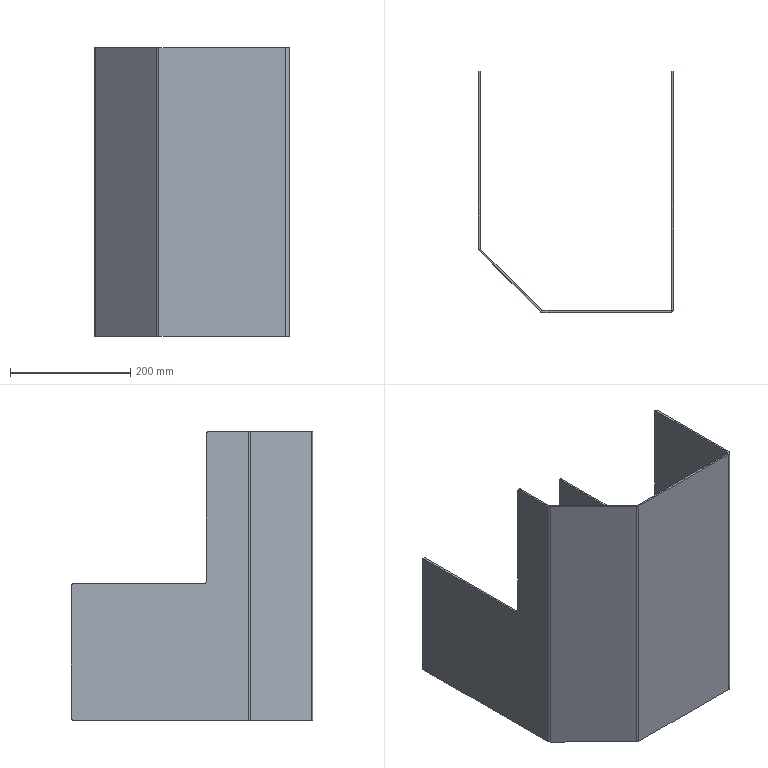Part | SolidWorks | features EdgeFlange 3, FlatPattern 1, SMBaseFlange 1, SheetMetal 1 | 1 solid | 46 faces | box 325 x 402 x 480 mm | volume 1150314 mm3 | plane 28 | cylinder 18 | commonest cylinder face diameters 6 x9 12 x5 8.5 x2 120 x2
STEP:
#1=CARTESIAN_POINT('',(325.,45.,-80.));
#2=VERTEX_POINT('',#1);
#3=CARTESIAN_POINT('',(325.,165.,-80.));
#4=VERTEX_POINT('',#3);
#5=CARTESIAN_POINT('',(325.,105.,-80.));
#6=DIRECTION('',(1.,0.,0.));
#7=DIRECTION('',(0.,1.,0.));
#8=AXIS2_PLACEMENT_3D('',#5,#6,#7);
#9=CIRCLE('',#8,60.);
#10=EDGE_CURVE('',#2,#4,#9,.T.);
#11=ORIENTED_EDGE('',*,*,#10,.T.);
#12=CARTESIAN_POINT('',(322.,165.,-80.));
#13=VERTEX_POINT('',#12);
#14=CARTESIAN_POINT('',(325.,165.,-80.));
#15=DIRECTION('',(-1.,0.,0.));
#16=VECTOR('',#15,1000.);
#17=LINE('',#14,#16);
#18=EDGE_CURVE('',#4,#13,#17,.T.);
#19=ORIENTED_EDGE('',*,*,#18,.T.);
#20=CARTESIAN_POINT('',(322.,45.,-80.));
#21=VERTEX_POINT('',#20);
#22=CARTESIAN_POINT('',(322.,105.,-80.));
#23=DIRECTION('',(1.,0.,0.));
#24=DIRECTION('',(0.,1.,0.));
#25=AXIS2_PLACEMENT_3D('',#22,#23,#24);
#26=CIRCLE('',#25,60.);
#27=EDGE_CURVE('',#21,#13,#26,.T.);
#28=ORIENTED_EDGE('',*,*,#27,.F.);
#29=CARTESIAN_POINT('',(325.,45.,-80.));
#30=DIRECTION('',(-1.,0.,0.));
#31=VECTOR('',#30,1000.);
#32=LINE('',#29,#31);
#33=EDGE_CURVE('',#2,#21,#32,.T.);
#34=ORIENTED_EDGE('',*,*,#33,.F.);
#35=EDGE_LOOP('',(#11,#19,#28,#34));
#36=FACE_OUTER_BOUND('',#35,.T.);
#37=CARTESIAN_POINT('',(325.,105.,-80.));
#38=DIRECTION('',(-1.,0.,0.));
#39=DIRECTION('',(0.,-1.,0.));
#40=AXIS2_PLACEMENT_3D('',#37,#38,#39);
#41=CYLINDRICAL_SURFACE('',#40,60.);
#42=ADVANCED_FACE('',(#36),#41,.F.);
#43=CARTESIAN_POINT('',(325.,25.75,210.));
#44=VERTEX_POINT('',#43);
#45=CARTESIAN_POINT('',(325.,34.25,210.));
#46=VERTEX_POINT('',#45);
#47=CARTESIAN_POINT('',(325.,30.,210.));
#48=DIRECTION('',(1.,0.,0.));
#49=DIRECTION('',(0.,1.,0.));
#50=AXIS2_PLACEMENT_3D('',#47,#48,#49);
#51=CIRCLE('',#50,4.25);
#52=EDGE_CURVE('',#44,#46,#51,.T.);
#53=ORIENTED_EDGE('',*,*,#52,.T.);
#54=CARTESIAN_POINT('',(322.,34.25,210.));
#55=VERTEX_POINT('',#54);
#56=CARTESIAN_POINT('',(325.,34.25,210.));
#57=DIRECTION('',(-1.,0.,0.));
#58=VECTOR('',#57,1000.);
#59=LINE('',#56,#58);
#60=EDGE_CURVE('',#46,#55,#59,.T.);
#61=ORIENTED_EDGE('',*,*,#60,.T.);
#62=CARTESIAN_POINT('',(322.,25.75,210.));
#63=VERTEX_POINT('',#62);
#64=CARTESIAN_POINT('',(322.,30.,210.));
#65=DIRECTION('',(1.,0.,0.));
#66=DIRECTION('',(0.,1.,0.));
#67=AXIS2_PLACEMENT_3D('',#64,#65,#66);
#68=CIRCLE('',#67,4.25);
#69=EDGE_CURVE('',#63,#55,#68,.T.);
#70=ORIENTED_EDGE('',*,*,#69,.F.);
#71=CARTESIAN_POINT('',(325.,25.75,210.));
#72=DIRECTION('',(-1.,0.,0.));
#73=VECTOR('',#72,1000.);
#74=LINE('',#71,#73);
#75=EDGE_CURVE('',#44,#63,#74,.T.);
#76=ORIENTED_EDGE('',*,*,#75,.F.);
#77=EDGE_LOOP('',(#53,#61,#70,#76));
#78=FACE_OUTER_BOUND('',#77,.T.);
#79=CARTESIAN_POINT('',(325.,30.,210.));
#80=DIRECTION('',(-1.,0.,0.));
#81=DIRECTION('',(0.,-1.,0.));
#82=AXIS2_PLACEMENT_3D('',#79,#80,#81);
#83=CYLINDRICAL_SURFACE('',#82,4.25);
#84=ADVANCED_FACE('',(#78),#83,.F.);
#85=CARTESIAN_POINT('',(319.,3.,-240.));
#86=VERTEX_POINT('',#85);
#87=CARTESIAN_POINT('',(107.485,3.,-240.));
#88=VERTEX_POINT('',#87);
#89=CARTESIAN_POINT('',(319.,3.,-240.));
#90=DIRECTION('',(-1.,0.,0.));
#91=VECTOR('',#90,1000.);
#92=LINE('',#89,#91);
#93=EDGE_CURVE('',#86,#88,#92,.T.);
#94=ORIENTED_EDGE('',*,*,#93,.F.);
#95=CARTESIAN_POINT('',(319.,0.,-240.));
#96=VERTEX_POINT('',#95);
#97=CARTESIAN_POINT('',(319.,0.,-240.));
#98=DIRECTION('',(0.,1.,0.));
#99=VECTOR('',#98,1000.);
#100=LINE('',#97,#99);
#101=EDGE_CURVE('',#96,#86,#100,.T.);
#102=ORIENTED_EDGE('',*,*,#101,.F.);
#103=CARTESIAN_POINT('',(107.485,0.,-240.));
#104=VERTEX_POINT('',#103);
#105=CARTESIAN_POINT('',(319.,0.,-240.));
#106=DIRECTION('',(-1.,0.,0.));
#107=VECTOR('',#106,1000.);
#108=LINE('',#105,#107);
#109=EDGE_CURVE('',#96,#104,#108,.T.);
#110=ORIENTED_EDGE('',*,*,#109,.T.);
#111=CARTESIAN_POINT('',(107.485,0.,-240.));
#112=DIRECTION('',(0.,1.,0.));
#113=VECTOR('',#112,1000.);
#114=LINE('',#111,#113);
#115=EDGE_CURVE('',#104,#88,#114,.T.);
#116=ORIENTED_EDGE('',*,*,#115,.T.);
#117=EDGE_LOOP('',(#94,#102,#110,#116));
#118=FACE_OUTER_BOUND('',#117,.T.);
#119=CARTESIAN_POINT('',(319.,0.,-240.));
#120=DIRECTION('',(0.,0.,-1.));
#121=DIRECTION('',(-1.,0.,0.));
#122=AXIS2_PLACEMENT_3D('',#119,#120,#121);
#123=PLANE('',#122);
#124=ADVANCED_FACE('',(#118),#123,.T.);
#125=CARTESIAN_POINT('',(107.485,3.,240.));
#126=VERTEX_POINT('',#125);
#127=CARTESIAN_POINT('',(319.,3.,240.));
#128=VERTEX_POINT('',#127);
#129=CARTESIAN_POINT('',(107.485,3.,240.));
#130=DIRECTION('',(1.,0.,0.));
#131=VECTOR('',#130,1000.);
#132=LINE('',#129,#131);
#133=EDGE_CURVE('',#126,#128,#132,.T.);
#134=ORIENTED_EDGE('',*,*,#133,.F.);
#135=CARTESIAN_POINT('',(107.485,0.,240.));
#136=VERTEX_POINT('',#135);
#137=CARTESIAN_POINT('',(107.485,0.,240.));
#138=DIRECTION('',(0.,1.,0.));
#139=VECTOR('',#138,1000.);
#140=LINE('',#137,#139);
#141=EDGE_CURVE('',#136,#126,#140,.T.);
#142=ORIENTED_EDGE('',*,*,#141,.F.);
#143=CARTESIAN_POINT('',(319.,0.,240.));
#144=VERTEX_POINT('',#143);
#145=CARTESIAN_POINT('',(107.485,0.,240.));
#146=DIRECTION('',(1.,0.,0.));
#147=VECTOR('',#146,1000.);
#148=LINE('',#145,#147);
#149=EDGE_CURVE('',#136,#144,#148,.T.);
#150=ORIENTED_EDGE('',*,*,#149,.T.);
#151=CARTESIAN_POINT('',(319.,0.,240.));
#152=DIRECTION('',(0.,1.,0.));
#153=VECTOR('',#152,1000.);
#154=LINE('',#151,#153);
#155=EDGE_CURVE('',#144,#128,#154,.T.);
#156=ORIENTED_EDGE('',*,*,#155,.T.);
#157=EDGE_LOOP('',(#134,#142,#150,#156));
#158=FACE_OUTER_BOUND('',#157,.T.);
#159=CARTESIAN_POINT('',(107.485,0.,240.));
#160=DIRECTION('',(0.,0.,1.));
#161=DIRECTION('',(1.,0.,0.));
#162=AXIS2_PLACEMENT_3D('',#159,#160,#161);
#163=PLANE('',#162);
#164=ADVANCED_FACE('',(#158),#163,.T.);
#165=ORIENTED_EDGE('',*,*,#109,.F.);
#166=CARTESIAN_POINT('',(319.,0.,240.));
#167=DIRECTION('',(0.,0.,-1.));
#168=VECTOR('',#167,1000.);
#169=LINE('',#166,#168);
#170=EDGE_CURVE('',#144,#96,#169,.T.);
#171=ORIENTED_EDGE('',*,*,#170,.F.);
#172=ORIENTED_EDGE('',*,*,#149,.F.);
#173=CARTESIAN_POINT('',(107.485,0.,-240.));
#174=DIRECTION('',(0.,0.,1.));
#175=VECTOR('',#174,1000.);
#176=LINE('',#173,#175);
#177=EDGE_CURVE('',#104,#136,#176,.T.);
#178=ORIENTED_EDGE('',*,*,#177,.F.);
#179=EDGE_LOOP('',(#165,#171,#172,#178));
#180=FACE_OUTER_BOUND('',#179,.T.);
#181=CARTESIAN_POINT('',(0.,0.,0.));
#182=DIRECTION('',(0.,1.,0.));
#183=DIRECTION('',(0.,0.,1.));
#184=AXIS2_PLACEMENT_3D('',#181,#182,#183);
#185=PLANE('',#184);
#186=ADVANCED_FACE('',(#180),#185,.F.);
#187=ORIENTED_EDGE('',*,*,#93,.T.);
#188=CARTESIAN_POINT('',(107.485,3.,-240.));
#189=DIRECTION('',(0.,0.,1.));
#190=VECTOR('',#189,1000.);
#191=LINE('',#188,#190);
#192=EDGE_CURVE('',#88,#126,#191,.T.);
#193=ORIENTED_EDGE('',*,*,#192,.T.);
#194=ORIENTED_EDGE('',*,*,#133,.T.);
#195=CARTESIAN_POINT('',(319.,3.,240.));
#196=DIRECTION('',(0.,0.,-1.));
#197=VECTOR('',#196,1000.);
#198=LINE('',#195,#197);
#199=EDGE_CURVE('',#128,#86,#198,.T.);
#200=ORIENTED_EDGE('',*,*,#199,.T.);
#201=EDGE_LOOP('',(#187,#193,#194,#200));
#202=FACE_OUTER_BOUND('',#201,.T.);
#203=CARTESIAN_POINT('',(0.,3.,0.));
#204=DIRECTION('',(0.,1.,0.));
#205=DIRECTION('',(0.,0.,1.));
#206=AXIS2_PLACEMENT_3D('',#203,#204,#205);
#207=PLANE('',#206);
#208=ADVANCED_FACE('',(#202),#207,.T.);
#209=CARTESIAN_POINT('',(105.364,3.879,-240.));
#210=VERTEX_POINT('',#209);
#211=CARTESIAN_POINT('',(103.243,1.757,-240.));
#212=VERTEX_POINT('',#211);
#213=CARTESIAN_POINT('',(103.243,1.757,-240.));
#214=DIRECTION('',(-0.7071,-0.7071,0.));
#215=VECTOR('',#214,1000.);
#216=LINE('',#213,#215);
#217=EDGE_CURVE('',#210,#212,#216,.T.);
#218=ORIENTED_EDGE('',*,*,#217,.F.);
#219=CARTESIAN_POINT('',(107.485,6.,-240.));
#220=DIRECTION('',(0.,0.,-1.));
#221=DIRECTION('',(1.,0.,0.));
#222=AXIS2_PLACEMENT_3D('',#219,#220,#221);
#223=CIRCLE('',#222,3.);
#224=EDGE_CURVE('',#88,#210,#223,.T.);
#225=ORIENTED_EDGE('',*,*,#224,.F.);
#226=ORIENTED_EDGE('',*,*,#115,.F.);
#227=CARTESIAN_POINT('',(107.485,6.,-240.));
#228=DIRECTION('',(0.,0.,-1.));
#229=DIRECTION('',(1.,0.,0.));
#230=AXIS2_PLACEMENT_3D('',#227,#228,#229);
#231=CIRCLE('',#230,6.);
#232=EDGE_CURVE('',#104,#212,#231,.T.);
#233=ORIENTED_EDGE('',*,*,#232,.T.);
#234=EDGE_LOOP('',(#218,#225,#226,#233));
#235=FACE_OUTER_BOUND('',#234,.T.);
#236=CARTESIAN_POINT('',(107.485,6.,-240.));
#237=DIRECTION('',(0.,0.,-1.));
#238=DIRECTION('',(-1.,0.,0.));
#239=AXIS2_PLACEMENT_3D('',#236,#237,#238);
#240=PLANE('',#239);
#241=ADVANCED_FACE('',(#235),#240,.T.);
#242=CARTESIAN_POINT('',(105.364,3.879,240.));
#243=VERTEX_POINT('',#242);
#244=CARTESIAN_POINT('',(107.485,6.,240.));
#245=DIRECTION('',(0.,0.,1.));
#246=DIRECTION('',(1.,0.,0.));
#247=AXIS2_PLACEMENT_3D('',#244,#245,#246);
#248=CIRCLE('',#247,3.);
#249=EDGE_CURVE('',#243,#126,#248,.T.);
#250=ORIENTED_EDGE('',*,*,#249,.F.);
#251=CARTESIAN_POINT('',(103.243,1.757,240.));
#252=VERTEX_POINT('',#251);
#253=CARTESIAN_POINT('',(105.364,3.879,240.));
#254=DIRECTION('',(-0.7071,-0.7071,0.));
#255=VECTOR('',#254,1000.);
#256=LINE('',#253,#255);
#257=EDGE_CURVE('',#243,#252,#256,.T.);
#258=ORIENTED_EDGE('',*,*,#257,.T.);
#259=CARTESIAN_POINT('',(107.485,6.,240.));
#260=DIRECTION('',(0.,0.,1.));
#261=DIRECTION('',(1.,0.,0.));
#262=AXIS2_PLACEMENT_3D('',#259,#260,#261);
#263=CIRCLE('',#262,6.);
#264=EDGE_CURVE('',#252,#136,#263,.T.);
#265=ORIENTED_EDGE('',*,*,#264,.T.);
#266=ORIENTED_EDGE('',*,*,#141,.T.);
#267=EDGE_LOOP('',(#250,#258,#265,#266));
#268=FACE_OUTER_BOUND('',#267,.T.);
#269=CARTESIAN_POINT('',(107.485,6.,240.));
#270=DIRECTION('',(0.,0.,-1.));
#271=DIRECTION('',(-1.,0.,0.));
#272=AXIS2_PLACEMENT_3D('',#269,#270,#271);
#273=PLANE('',#272);
#274=ADVANCED_FACE('',(#268),#273,.F.);
#275=ORIENTED_EDGE('',*,*,#177,.T.);
#276=ORIENTED_EDGE('',*,*,#264,.F.);
#277=CARTESIAN_POINT('',(103.243,1.757,-240.));
#278=DIRECTION('',(0.,0.,-1.));
#279=VECTOR('',#278,1000.);
#280=LINE('',#277,#279);
#281=EDGE_CURVE('',#252,#212,#280,.T.);
#282=ORIENTED_EDGE('',*,*,#281,.T.);
#283=ORIENTED_EDGE('',*,*,#232,.F.);
#284=EDGE_LOOP('',(#275,#276,#282,#283));
#285=FACE_OUTER_BOUND('',#284,.T.);
#286=CARTESIAN_POINT('',(107.485,6.,240.));
#287=DIRECTION('',(0.,0.,1.));
#288=DIRECTION('',(-0.7071,-0.7071,0.));
#289=AXIS2_PLACEMENT_3D('',#286,#287,#288);
#290=CYLINDRICAL_SURFACE('',#289,6.);
#291=ADVANCED_FACE('',(#285),#290,.T.);
#292=ORIENTED_EDGE('',*,*,#192,.F.);
#293=ORIENTED_EDGE('',*,*,#224,.T.);
#294=CARTESIAN_POINT('',(105.364,3.879,-240.));
#295=DIRECTION('',(0.,0.,1.));
#296=VECTOR('',#295,1000.);
#297=LINE('',#294,#296);
#298=EDGE_CURVE('',#210,#243,#297,.T.);
#299=ORIENTED_EDGE('',*,*,#298,.T.);
#300=ORIENTED_EDGE('',*,*,#249,.T.);
#301=EDGE_LOOP('',(#292,#293,#299,#300));
#302=FACE_OUTER_BOUND('',#301,.T.);
#303=CARTESIAN_POINT('',(107.485,6.,240.));
#304=DIRECTION('',(0.,0.,1.));
#305=DIRECTION('',(-0.7071,-0.7071,0.));
#306=AXIS2_PLACEMENT_3D('',#303,#304,#305);
#307=CYLINDRICAL_SURFACE('',#306,3.);
#308=ADVANCED_FACE('',(#302),#307,.F.);
#309=ORIENTED_EDGE('',*,*,#257,.F.);
#310=CARTESIAN_POINT('',(3.879,105.364,240.));
#311=VERTEX_POINT('',#310);
#312=CARTESIAN_POINT('',(3.879,105.364,240.));
#313=DIRECTION('',(-0.7071,0.7071,0.));
#314=VECTOR('',#313,1000.);
#315=LINE('',#312,#314);
#316=EDGE_CURVE('',#243,#311,#315,.T.);
#317=ORIENTED_EDGE('',*,*,#316,.T.);
#318=CARTESIAN_POINT('',(1.757,103.243,240.));
#319=VERTEX_POINT('',#318);
#320=CARTESIAN_POINT('',(1.757,103.243,240.));
#321=DIRECTION('',(0.7071,0.7071,0.));
#322=VECTOR('',#321,1000.);
#323=LINE('',#320,#322);
#324=EDGE_CURVE('',#319,#311,#323,.T.);
#325=ORIENTED_EDGE('',*,*,#324,.F.);
#326=CARTESIAN_POINT('',(51.879,53.121,240.));
#327=DIRECTION('',(-0.7071,0.7071,0.));
#328=VECTOR('',#327,1000.);
#329=LINE('',#326,#328);
#330=EDGE_CURVE('',#252,#319,#329,.T.);
#331=ORIENTED_EDGE('',*,*,#330,.F.);
#332=EDGE_LOOP('',(#309,#317,#325,#331));
#333=FACE_OUTER_BOUND('',#332,.T.);
#334=CARTESIAN_POINT('',(1.757,103.243,240.));
#335=DIRECTION('',(0.,0.,-1.));
#336=DIRECTION('',(-1.,0.,0.));
#337=AXIS2_PLACEMENT_3D('',#334,#335,#336);
#338=PLANE('',#337);
#339=ADVANCED_FACE('',(#333),#338,.F.);
#340=ORIENTED_EDGE('',*,*,#217,.T.);
#341=CARTESIAN_POINT('',(1.757,103.243,-240.));
#342=VERTEX_POINT('',#341);
#343=CARTESIAN_POINT('',(51.879,53.121,-240.));
#344=DIRECTION('',(0.7071,-0.7071,0.));
#345=VECTOR('',#344,1000.);
#346=LINE('',#343,#345);
#347=EDGE_CURVE('',#342,#212,#346,.T.);
#348=ORIENTED_EDGE('',*,*,#347,.F.);
#349=CARTESIAN_POINT('',(3.879,105.364,-240.));
#350=VERTEX_POINT('',#349);
#351=CARTESIAN_POINT('',(1.757,103.243,-240.));
#352=DIRECTION('',(0.7071,0.7071,0.));
#353=VECTOR('',#352,1000.);
#354=LINE('',#351,#353);
#355=EDGE_CURVE('',#342,#350,#354,.T.);
#356=ORIENTED_EDGE('',*,*,#355,.T.);
#357=CARTESIAN_POINT('',(106.243,3.,-240.));
#358=DIRECTION('',(0.7071,-0.7071,0.));
#359=VECTOR('',#358,1000.);
#360=LINE('',#357,#359);
#361=EDGE_CURVE('',#350,#210,#360,.T.);
#362=ORIENTED_EDGE('',*,*,#361,.T.);
#363=EDGE_LOOP('',(#340,#348,#356,#362));
#364=FACE_OUTER_BOUND('',#363,.T.);
#365=CARTESIAN_POINT('',(104.121,0.8787,-240.));
#366=DIRECTION('',(0.,0.,1.));
#367=DIRECTION('',(1.,0.,0.));
#368=AXIS2_PLACEMENT_3D('',#365,#366,#367);
#369=PLANE('',#368);
#370=ADVANCED_FACE('',(#364),#369,.F.);
#371=ORIENTED_EDGE('',*,*,#281,.F.);
#372=ORIENTED_EDGE('',*,*,#330,.T.);
#373=CARTESIAN_POINT('',(1.757,103.243,0.));
#374=DIRECTION('',(0.,0.,-1.));
#375=VECTOR('',#374,1000.);
#376=LINE('',#373,#375);
#377=EDGE_CURVE('',#319,#342,#376,.T.);
#378=ORIENTED_EDGE('',*,*,#377,.T.);
#379=ORIENTED_EDGE('',*,*,#347,.T.);
#380=EDGE_LOOP('',(#371,#372,#378,#379));
#381=FACE_OUTER_BOUND('',#380,.T.);
#382=CARTESIAN_POINT('',(51.879,53.121,0.));
#383=DIRECTION('',(0.7071,0.7071,0.));
#384=DIRECTION('',(-0.7071,0.7071,0.));
#385=AXIS2_PLACEMENT_3D('',#382,#383,#384);
#386=PLANE('',#385);
#387=ADVANCED_FACE('',(#381),#386,.F.);
#388=ORIENTED_EDGE('',*,*,#316,.F.);
#389=ORIENTED_EDGE('',*,*,#298,.F.);
#390=ORIENTED_EDGE('',*,*,#361,.F.);
#391=CARTESIAN_POINT('',(3.879,105.364,-240.));
#392=DIRECTION('',(0.,0.,-1.));
#393=VECTOR('',#392,1000.);
#394=LINE('',#391,#393);
#395=EDGE_CURVE('',#311,#350,#394,.T.);
#396=ORIENTED_EDGE('',*,*,#395,.F.);
#397=EDGE_LOOP('',(#388,#389,#390,#396));
#398=FACE_OUTER_BOUND('',#397,.T.);
#399=CARTESIAN_POINT('',(54.,55.243,0.));
#400=DIRECTION('',(0.7071,0.7071,0.));
#401=DIRECTION('',(-0.7071,0.7071,0.));
#402=AXIS2_PLACEMENT_3D('',#399,#400,#401);
#403=PLANE('',#402);
#404=ADVANCED_FACE('',(#398),#403,.T.);
#405=CARTESIAN_POINT('',(322.,6.,240.));
#406=VERTEX_POINT('',#405);
#407=CARTESIAN_POINT('',(325.,6.,240.));
#408=VERTEX_POINT('',#407);
#409=CARTESIAN_POINT('',(325.,6.,240.));
#410=DIRECTION('',(1.,0.,0.));
#411=VECTOR('',#410,1000.);
#412=LINE('',#409,#411);
#413=EDGE_CURVE('',#406,#408,#412,.T.);
#414=ORIENTED_EDGE('',*,*,#413,.F.);
#415=CARTESIAN_POINT('',(319.,6.,240.));
#416=DIRECTION('',(0.,0.,1.));
#417=DIRECTION('',(-1.,0.,0.));
#418=AXIS2_PLACEMENT_3D('',#415,#416,#417);
#419=CIRCLE('',#418,3.);
#420=EDGE_CURVE('',#128,#406,#419,.T.);
#421=ORIENTED_EDGE('',*,*,#420,.F.);
#422=ORIENTED_EDGE('',*,*,#155,.F.);
#423=CARTESIAN_POINT('',(319.,6.,240.));
#424=DIRECTION('',(0.,0.,1.));
#425=DIRECTION('',(-1.,0.,0.));
#426=AXIS2_PLACEMENT_3D('',#423,#424,#425);
#427=CIRCLE('',#426,6.);
#428=EDGE_CURVE('',#144,#408,#427,.T.);
#429=ORIENTED_EDGE('',*,*,#428,.T.);
#430=EDGE_LOOP('',(#414,#421,#422,#429));
#431=FACE_OUTER_BOUND('',#430,.T.);
#432=CARTESIAN_POINT('',(319.,6.,240.));
#433=DIRECTION('',(0.,0.,1.));
#434=DIRECTION('',(1.,0.,0.));
#435=AXIS2_PLACEMENT_3D('',#432,#433,#434);
#436=PLANE('',#435);
#437=ADVANCED_FACE('',(#431),#436,.T.);
#438=CARTESIAN_POINT('',(322.,6.,-240.));
#439=VERTEX_POINT('',#438);
#440=CARTESIAN_POINT('',(319.,6.,-240.));
#441=DIRECTION('',(0.,0.,-1.));
#442=DIRECTION('',(-1.,0.,0.));
#443=AXIS2_PLACEMENT_3D('',#440,#441,#442);
#444=CIRCLE('',#443,3.);
#445=EDGE_CURVE('',#439,#86,#444,.T.);
#446=ORIENTED_EDGE('',*,*,#445,.F.);
#447=CARTESIAN_POINT('',(325.,6.,-240.));
#448=VERTEX_POINT('',#447);
#449=CARTESIAN_POINT('',(322.,6.,-240.));
#450=DIRECTION('',(1.,0.,0.));
#451=VECTOR('',#450,1000.);
#452=LINE('',#449,#451);
#453=EDGE_CURVE('',#439,#448,#452,.T.);
#454=ORIENTED_EDGE('',*,*,#453,.T.);
#455=CARTESIAN_POINT('',(319.,6.,-240.));
#456=DIRECTION('',(0.,0.,-1.));
#457=DIRECTION('',(-1.,0.,0.));
#458=AXIS2_PLACEMENT_3D('',#455,#456,#457);
#459=CIRCLE('',#458,6.);
#460=EDGE_CURVE('',#448,#96,#459,.T.);
#461=ORIENTED_EDGE('',*,*,#460,.T.);
#462=ORIENTED_EDGE('',*,*,#101,.T.);
#463=EDGE_LOOP('',(#446,#454,#461,#462));
#464=FACE_OUTER_BOUND('',#463,.T.);
#465=CARTESIAN_POINT('',(319.,6.,-240.));
#466=DIRECTION('',(0.,0.,1.));
#467=DIRECTION('',(1.,0.,0.));
#468=AXIS2_PLACEMENT_3D('',#465,#466,#467);
#469=PLANE('',#468);
#470=ADVANCED_FACE('',(#464),#469,.F.);
#471=ORIENTED_EDGE('',*,*,#170,.T.);
#472=ORIENTED_EDGE('',*,*,#460,.F.);
#473=CARTESIAN_POINT('',(325.,6.,237.));
#474=DIRECTION('',(0.,0.,-1.));
#475=VECTOR('',#474,1000.);
#476=LINE('',#473,#475);
#477=EDGE_CURVE('',#408,#448,#476,.T.);
#478=ORIENTED_EDGE('',*,*,#477,.F.);
#479=ORIENTED_EDGE('',*,*,#428,.F.);
#480=EDGE_LOOP('',(#471,#472,#478,#479));
#481=FACE_OUTER_BOUND('',#480,.T.);
#482=CARTESIAN_POINT('',(319.,6.,-240.));
#483=DIRECTION('',(0.,0.,-1.));
#484=DIRECTION('',(1.,0.,0.));
#485=AXIS2_PLACEMENT_3D('',#482,#483,#484);
#486=CYLINDRICAL_SURFACE('',#485,6.);
#487=ADVANCED_FACE('',(#481),#486,.T.);
#488=ORIENTED_EDGE('',*,*,#199,.F.);
#489=ORIENTED_EDGE('',*,*,#420,.T.);
#490=CARTESIAN_POINT('',(322.,6.,240.));
#491=DIRECTION('',(0.,0.,-1.));
#492=VECTOR('',#491,1000.);
#493=LINE('',#490,#492);
#494=EDGE_CURVE('',#406,#439,#493,.T.);
#495=ORIENTED_EDGE('',*,*,#494,.T.);
#496=ORIENTED_EDGE('',*,*,#445,.T.);
#497=EDGE_LOOP('',(#488,#489,#495,#496));
#498=FACE_OUTER_BOUND('',#497,.T.);
#499=CARTESIAN_POINT('',(319.,6.,-240.));
#500=DIRECTION('',(0.,0.,-1.));
#501=DIRECTION('',(1.,0.,0.));
#502=AXIS2_PLACEMENT_3D('',#499,#500,#501);
#503=CYLINDRICAL_SURFACE('',#502,3.);
#504=ADVANCED_FACE('',(#498),#503,.F.);
#505=ORIENTED_EDGE('',*,*,#52,.F.);
#506=CARTESIAN_POINT('',(325.,30.,210.));
#507=DIRECTION('',(1.,0.,0.));
#508=DIRECTION('',(0.,1.,0.));
#509=AXIS2_PLACEMENT_3D('',#506,#507,#508);
#510=CIRCLE('',#509,4.25);
#511=EDGE_CURVE('',#46,#44,#510,.T.);
#512=ORIENTED_EDGE('',*,*,#511,.F.);
#513=EDGE_LOOP('',(#505,#512));
#514=FACE_BOUND('',#513,.T.);
#515=ORIENTED_EDGE('',*,*,#10,.F.);
#516=CARTESIAN_POINT('',(325.,105.,-80.));
#517=DIRECTION('',(1.,0.,0.));
#518=DIRECTION('',(0.,1.,0.));
#519=AXIS2_PLACEMENT_3D('',#516,#517,#518);
#520=CIRCLE('',#519,60.);
#521=EDGE_CURVE('',#4,#2,#520,.T.);
#522=ORIENTED_EDGE('',*,*,#521,.F.);
#523=EDGE_LOOP('',(#515,#522));
#524=FACE_BOUND('',#523,.T.);
#525=CARTESIAN_POINT('',(325.,174.,240.));
#526=VERTEX_POINT('',#525);
#527=CARTESIAN_POINT('',(325.,174.,240.));
#528=DIRECTION('',(0.,-1.,0.));
#529=VECTOR('',#528,1000.);
#530=LINE('',#527,#529);
#531=EDGE_CURVE('',#526,#408,#530,.T.);
#532=ORIENTED_EDGE('',*,*,#531,.T.);
#533=ORIENTED_EDGE('',*,*,#477,.T.);
#534=CARTESIAN_POINT('',(325.,399.,-240.));
#535=VERTEX_POINT('',#534);
#536=CARTESIAN_POINT('',(325.,174.,-240.));
#537=DIRECTION('',(0.,1.,0.));
#538=VECTOR('',#537,1000.);
#539=LINE('',#536,#538);
#540=EDGE_CURVE('',#448,#535,#539,.T.);
#541=ORIENTED_EDGE('',*,*,#540,.T.);
#542=CARTESIAN_POINT('',(325.,402.,-237.));
#543=VERTEX_POINT('',#542);
#544=CARTESIAN_POINT('',(325.,399.,-237.));
#545=DIRECTION('',(1.,0.,0.));
#546=DIRECTION('',(0.,1.,0.));
#547=AXIS2_PLACEMENT_3D('',#544,#545,#546);
#548=CIRCLE('',#547,3.);
#549=EDGE_CURVE('',#535,#543,#548,.T.);
#550=ORIENTED_EDGE('',*,*,#549,.T.);
#551=CARTESIAN_POINT('',(325.,402.,-16.));
#552=VERTEX_POINT('',#551);
#553=CARTESIAN_POINT('',(325.,402.,237.));
#554=DIRECTION('',(0.,0.,1.));
#555=VECTOR('',#554,1000.);
#556=LINE('',#553,#555);
#557=EDGE_CURVE('',#543,#552,#556,.T.);
#558=ORIENTED_EDGE('',*,*,#557,.T.);
#559=CARTESIAN_POINT('',(325.,399.,-13.));
#560=VERTEX_POINT('',#559);
#561=CARTESIAN_POINT('',(325.,399.,-16.));
#562=DIRECTION('',(1.,0.,0.));
#563=DIRECTION('',(0.,1.,0.));
#564=AXIS2_PLACEMENT_3D('',#561,#562,#563);
#565=CIRCLE('',#564,3.);
#566=EDGE_CURVE('',#552,#560,#565,.T.);
#567=ORIENTED_EDGE('',*,*,#566,.T.);
#568=CARTESIAN_POINT('',(325.,183.,-13.));
#569=VERTEX_POINT('',#568);
#570=CARTESIAN_POINT('',(325.,174.,-13.));
#571=DIRECTION('',(0.,-1.,0.));
#572=VECTOR('',#571,1000.);
#573=LINE('',#570,#572);
#574=EDGE_CURVE('',#560,#569,#573,.T.);
#575=ORIENTED_EDGE('',*,*,#574,.T.);
#576=CARTESIAN_POINT('',(325.,177.,-7.));
#577=VERTEX_POINT('',#576);
#578=CARTESIAN_POINT('',(325.,183.,-7.));
#579=DIRECTION('',(-1.,0.,0.));
#580=DIRECTION('',(0.,1.,0.));
#581=AXIS2_PLACEMENT_3D('',#578,#579,#580);
#582=CIRCLE('',#581,6.);
#583=EDGE_CURVE('',#569,#577,#582,.T.);
#584=ORIENTED_EDGE('',*,*,#583,.T.);
#585=CARTESIAN_POINT('',(325.,177.,237.));
#586=VERTEX_POINT('',#585);
#587=CARTESIAN_POINT('',(325.,177.,237.));
#588=DIRECTION('',(0.,0.,1.));
#589=VECTOR('',#588,1000.);
#590=LINE('',#587,#589);
#591=EDGE_CURVE('',#577,#586,#590,.T.);
#592=ORIENTED_EDGE('',*,*,#591,.T.);
#593=CARTESIAN_POINT('',(325.,174.,237.));
#594=DIRECTION('',(1.,0.,0.));
#595=DIRECTION('',(0.,1.,0.));
#596=AXIS2_PLACEMENT_3D('',#593,#594,#595);
#597=CIRCLE('',#596,3.);
#598=EDGE_CURVE('',#586,#526,#597,.T.);
#599=ORIENTED_EDGE('',*,*,#598,.T.);
#600=EDGE_LOOP('',(#532,#533,#541,#550,#558,#567,#575,#584,#592,#599));
#601=FACE_OUTER_BOUND('',#600,.T.);
#602=CARTESIAN_POINT('',(325.,174.,237.));
#603=DIRECTION('',(1.,0.,0.));
#604=DIRECTION('',(0.,1.,0.));
#605=AXIS2_PLACEMENT_3D('',#602,#603,#604);
#606=PLANE('',#605);
#607=ADVANCED_FACE('',(#514,#524,#601),#606,.T.);
#608=ORIENTED_EDGE('',*,*,#27,.T.);
#609=CARTESIAN_POINT('',(322.,105.,-80.));
#610=DIRECTION('',(1.,0.,0.));
#611=DIRECTION('',(0.,1.,0.));
#612=AXIS2_PLACEMENT_3D('',#609,#610,#611);
#613=CIRCLE('',#612,60.);
#614=EDGE_CURVE('',#13,#21,#613,.T.);
#615=ORIENTED_EDGE('',*,*,#614,.T.);
#616=EDGE_LOOP('',(#608,#615));
#617=FACE_BOUND('',#616,.T.);
#618=ORIENTED_EDGE('',*,*,#69,.T.);
#619=CARTESIAN_POINT('',(322.,30.,210.));
#620=DIRECTION('',(1.,0.,0.));
#621=DIRECTION('',(0.,1.,0.));
#622=AXIS2_PLACEMENT_3D('',#619,#620,#621);
#623=CIRCLE('',#622,4.25);
#624=EDGE_CURVE('',#55,#63,#623,.T.);
#625=ORIENTED_EDGE('',*,*,#624,.T.);
#626=EDGE_LOOP('',(#618,#625));
#627=FACE_BOUND('',#626,.T.);
#628=ORIENTED_EDGE('',*,*,#494,.F.);
#629=CARTESIAN_POINT('',(322.,174.,240.));
#630=VERTEX_POINT('',#629);
#631=CARTESIAN_POINT('',(322.,3.,240.));
#632=DIRECTION('',(0.,-1.,0.));
#633=VECTOR('',#632,1000.);
#634=LINE('',#631,#633);
#635=EDGE_CURVE('',#630,#406,#634,.T.);
#636=ORIENTED_EDGE('',*,*,#635,.F.);
#637=CARTESIAN_POINT('',(322.,177.,237.));
#638=VERTEX_POINT('',#637);
#639=CARTESIAN_POINT('',(322.,174.,237.));
#640=DIRECTION('',(1.,0.,0.));
#641=DIRECTION('',(0.,1.,0.));
#642=AXIS2_PLACEMENT_3D('',#639,#640,#641);
#643=CIRCLE('',#642,3.);
#644=EDGE_CURVE('',#638,#630,#643,.T.);
#645=ORIENTED_EDGE('',*,*,#644,.F.);
#646=CARTESIAN_POINT('',(322.,177.,-7.));
#647=VERTEX_POINT('',#646);
#648=CARTESIAN_POINT('',(322.,177.,237.));
#649=DIRECTION('',(0.,0.,1.));
#650=VECTOR('',#649,1000.);
#651=LINE('',#648,#650);
#652=EDGE_CURVE('',#647,#638,#651,.T.);
#653=ORIENTED_EDGE('',*,*,#652,.F.);
#654=CARTESIAN_POINT('',(322.,183.,-13.));
#655=VERTEX_POINT('',#654);
#656=CARTESIAN_POINT('',(322.,183.,-7.));
#657=DIRECTION('',(-1.,0.,0.));
#658=DIRECTION('',(0.,1.,0.));
#659=AXIS2_PLACEMENT_3D('',#656,#657,#658);
#660=CIRCLE('',#659,6.);
#661=EDGE_CURVE('',#655,#647,#660,.T.);
#662=ORIENTED_EDGE('',*,*,#661,.F.);
#663=CARTESIAN_POINT('',(322.,399.,-13.));
#664=VERTEX_POINT('',#663);
#665=CARTESIAN_POINT('',(322.,183.,-13.));
#666=DIRECTION('',(0.,-1.,0.));
#667=VECTOR('',#666,1000.);
#668=LINE('',#665,#667);
#669=EDGE_CURVE('',#664,#655,#668,.T.);
#670=ORIENTED_EDGE('',*,*,#669,.F.);
#671=CARTESIAN_POINT('',(322.,402.,-16.));
#672=VERTEX_POINT('',#671);
#673=CARTESIAN_POINT('',(322.,399.,-16.));
#674=DIRECTION('',(1.,0.,0.));
#675=DIRECTION('',(0.,1.,0.));
#676=AXIS2_PLACEMENT_3D('',#673,#674,#675);
#677=CIRCLE('',#676,3.);
#678=EDGE_CURVE('',#672,#664,#677,.T.);
#679=ORIENTED_EDGE('',*,*,#678,.F.);
#680=CARTESIAN_POINT('',(322.,402.,-237.));
#681=VERTEX_POINT('',#680);
#682=CARTESIAN_POINT('',(322.,402.,-16.));
#683=DIRECTION('',(0.,0.,1.));
#684=VECTOR('',#683,1000.);
#685=LINE('',#682,#684);
#686=EDGE_CURVE('',#681,#672,#685,.T.);
#687=ORIENTED_EDGE('',*,*,#686,.F.);
#688=CARTESIAN_POINT('',(322.,399.,-240.));
#689=VERTEX_POINT('',#688);
#690=CARTESIAN_POINT('',(322.,399.,-237.));
#691=DIRECTION('',(1.,0.,0.));
#692=DIRECTION('',(0.,1.,0.));
#693=AXIS2_PLACEMENT_3D('',#690,#691,#692);
#694=CIRCLE('',#693,3.);
#695=EDGE_CURVE('',#689,#681,#694,.T.);
#696=ORIENTED_EDGE('',*,*,#695,.F.);
#697=CARTESIAN_POINT('',(322.,399.,-240.));
#698=DIRECTION('',(0.,1.,0.));
#699=VECTOR('',#698,1000.);
#700=LINE('',#697,#699);
#701=EDGE_CURVE('',#439,#689,#700,.T.);
#702=ORIENTED_EDGE('',*,*,#701,.F.);
#703=EDGE_LOOP('',(#628,#636,#645,#653,#662,#670,#679,#687,#696,#702));
#704=FACE_OUTER_BOUND('',#703,.T.);
#705=CARTESIAN_POINT('',(322.,174.,237.));
#706=DIRECTION('',(1.,0.,0.));
#707=DIRECTION('',(0.,1.,0.));
#708=AXIS2_PLACEMENT_3D('',#705,#706,#707);
#709=PLANE('',#708);
#710=ADVANCED_FACE('',(#617,#627,#704),#709,.F.);
#711=ORIENTED_EDGE('',*,*,#453,.F.);
#712=ORIENTED_EDGE('',*,*,#701,.T.);
#713=CARTESIAN_POINT('',(325.,399.,-240.));
#714=DIRECTION('',(-1.,0.,0.));
#715=VECTOR('',#714,1000.);
#716=LINE('',#713,#715);
#717=EDGE_CURVE('',#535,#689,#716,.T.);
#718=ORIENTED_EDGE('',*,*,#717,.F.);
#719=ORIENTED_EDGE('',*,*,#540,.F.);
#720=EDGE_LOOP('',(#711,#712,#718,#719));
#721=FACE_OUTER_BOUND('',#720,.T.);
#722=CARTESIAN_POINT('',(325.,399.,-240.));
#723=DIRECTION('',(0.,0.,1.));
#724=DIRECTION('',(1.,0.,0.));
#725=AXIS2_PLACEMENT_3D('',#722,#723,#724);
#726=PLANE('',#725);
#727=ADVANCED_FACE('',(#721),#726,.F.);
#728=ORIENTED_EDGE('',*,*,#413,.T.);
#729=ORIENTED_EDGE('',*,*,#531,.F.);
#730=CARTESIAN_POINT('',(325.,174.,240.));
#731=DIRECTION('',(-1.,0.,0.));
#732=VECTOR('',#731,1000.);
#733=LINE('',#730,#732);
#734=EDGE_CURVE('',#526,#630,#733,.T.);
#735=ORIENTED_EDGE('',*,*,#734,.T.);
#736=ORIENTED_EDGE('',*,*,#635,.T.);
#737=EDGE_LOOP('',(#728,#729,#735,#736));
#738=FACE_OUTER_BOUND('',#737,.T.);
#739=CARTESIAN_POINT('',(325.,3.,240.));
#740=DIRECTION('',(0.,0.,-1.));
#741=DIRECTION('',(-1.,0.,0.));
#742=AXIS2_PLACEMENT_3D('',#739,#740,#741);
#743=PLANE('',#742);
#744=ADVANCED_FACE('',(#738),#743,.F.);
#745=ORIENTED_EDGE('',*,*,#695,.T.);
#746=CARTESIAN_POINT('',(325.,402.,-237.));
#747=DIRECTION('',(-1.,0.,0.));
#748=VECTOR('',#747,1000.);
#749=LINE('',#746,#748);
#750=EDGE_CURVE('',#543,#681,#749,.T.);
#751=ORIENTED_EDGE('',*,*,#750,.F.);
#752=ORIENTED_EDGE('',*,*,#549,.F.);
#753=ORIENTED_EDGE('',*,*,#717,.T.);
#754=EDGE_LOOP('',(#745,#751,#752,#753));
#755=FACE_OUTER_BOUND('',#754,.T.);
#756=CARTESIAN_POINT('',(325.,399.,-237.));
#757=DIRECTION('',(-1.,0.,0.));
#758=DIRECTION('',(0.,-1.,0.));
#759=AXIS2_PLACEMENT_3D('',#756,#757,#758);
#760=CYLINDRICAL_SURFACE('',#759,3.);
#761=ADVANCED_FACE('',(#755),#760,.T.);
#762=ORIENTED_EDGE('',*,*,#686,.T.);
#763=CARTESIAN_POINT('',(325.,402.,-16.));
#764=DIRECTION('',(-1.,0.,0.));
#765=VECTOR('',#764,1000.);
#766=LINE('',#763,#765);
#767=EDGE_CURVE('',#552,#672,#766,.T.);
#768=ORIENTED_EDGE('',*,*,#767,.F.);
#769=ORIENTED_EDGE('',*,*,#557,.F.);
#770=ORIENTED_EDGE('',*,*,#750,.T.);
#771=EDGE_LOOP('',(#762,#768,#769,#770));
#772=FACE_OUTER_BOUND('',#771,.T.);
#773=CARTESIAN_POINT('',(325.,402.,-16.));
#774=DIRECTION('',(0.,-1.,0.));
#775=DIRECTION('',(1.,0.,0.));
#776=AXIS2_PLACEMENT_3D('',#773,#774,#775);
#777=PLANE('',#776);
#778=ADVANCED_FACE('',(#772),#777,.F.);
#779=ORIENTED_EDGE('',*,*,#678,.T.);
#780=CARTESIAN_POINT('',(325.,399.,-13.));
#781=DIRECTION('',(-1.,0.,0.));
#782=VECTOR('',#781,1000.);
#783=LINE('',#780,#782);
#784=EDGE_CURVE('',#560,#664,#783,.T.);
#785=ORIENTED_EDGE('',*,*,#784,.F.);
#786=ORIENTED_EDGE('',*,*,#566,.F.);
#787=ORIENTED_EDGE('',*,*,#767,.T.);
#788=EDGE_LOOP('',(#779,#785,#786,#787));
#789=FACE_OUTER_BOUND('',#788,.T.);
#790=CARTESIAN_POINT('',(325.,399.,-16.));
#791=DIRECTION('',(-1.,0.,0.));
#792=DIRECTION('',(0.,-1.,0.));
#793=AXIS2_PLACEMENT_3D('',#790,#791,#792);
#794=CYLINDRICAL_SURFACE('',#793,3.);
#795=ADVANCED_FACE('',(#789),#794,.T.);
#796=ORIENTED_EDGE('',*,*,#669,.T.);
#797=CARTESIAN_POINT('',(325.,183.,-13.));
#798=DIRECTION('',(-1.,0.,0.));
#799=VECTOR('',#798,1000.);
#800=LINE('',#797,#799);
#801=EDGE_CURVE('',#569,#655,#800,.T.);
#802=ORIENTED_EDGE('',*,*,#801,.F.);
#803=ORIENTED_EDGE('',*,*,#574,.F.);
#804=ORIENTED_EDGE('',*,*,#784,.T.);
#805=EDGE_LOOP('',(#796,#802,#803,#804));
#806=FACE_OUTER_BOUND('',#805,.T.);
#807=CARTESIAN_POINT('',(325.,183.,-13.));
#808=DIRECTION('',(0.,0.,-1.));
#809=DIRECTION('',(-1.,0.,0.));
#810=AXIS2_PLACEMENT_3D('',#807,#808,#809);
#811=PLANE('',#810);
#812=ADVANCED_FACE('',(#806),#811,.F.);
#813=ORIENTED_EDGE('',*,*,#661,.T.);
#814=CARTESIAN_POINT('',(325.,177.,-7.));
#815=DIRECTION('',(-1.,0.,0.));
#816=VECTOR('',#815,1000.);
#817=LINE('',#814,#816);
#818=EDGE_CURVE('',#577,#647,#817,.T.);
#819=ORIENTED_EDGE('',*,*,#818,.F.);
#820=ORIENTED_EDGE('',*,*,#583,.F.);
#821=ORIENTED_EDGE('',*,*,#801,.T.);
#822=EDGE_LOOP('',(#813,#819,#820,#821));
#823=FACE_OUTER_BOUND('',#822,.T.);
#824=CARTESIAN_POINT('',(325.,183.,-7.));
#825=DIRECTION('',(-1.,0.,0.));
#826=DIRECTION('',(0.,-1.,0.));
#827=AXIS2_PLACEMENT_3D('',#824,#825,#826);
#828=CYLINDRICAL_SURFACE('',#827,6.);
#829=ADVANCED_FACE('',(#823),#828,.F.);
#830=ORIENTED_EDGE('',*,*,#652,.T.);
#831=CARTESIAN_POINT('',(325.,177.,237.));
#832=DIRECTION('',(-1.,0.,0.));
#833=VECTOR('',#832,1000.);
#834=LINE('',#831,#833);
#835=EDGE_CURVE('',#586,#638,#834,.T.);
#836=ORIENTED_EDGE('',*,*,#835,.F.);
#837=ORIENTED_EDGE('',*,*,#591,.F.);
#838=ORIENTED_EDGE('',*,*,#818,.T.);
#839=EDGE_LOOP('',(#830,#836,#837,#838));
#840=FACE_OUTER_BOUND('',#839,.T.);
#841=CARTESIAN_POINT('',(325.,177.,237.));
#842=DIRECTION('',(0.,-1.,0.));
#843=DIRECTION('',(1.,0.,0.));
#844=AXIS2_PLACEMENT_3D('',#841,#842,#843);
#845=PLANE('',#844);
#846=ADVANCED_FACE('',(#840),#845,.F.);
#847=ORIENTED_EDGE('',*,*,#644,.T.);
#848=ORIENTED_EDGE('',*,*,#734,.F.);
#849=ORIENTED_EDGE('',*,*,#598,.F.);
#850=ORIENTED_EDGE('',*,*,#835,.T.);
#851=EDGE_LOOP('',(#847,#848,#849,#850));
#852=FACE_OUTER_BOUND('',#851,.T.);
#853=CARTESIAN_POINT('',(325.,174.,237.));
#854=DIRECTION('',(-1.,0.,0.));
#855=DIRECTION('',(0.,-1.,0.));
#856=AXIS2_PLACEMENT_3D('',#853,#854,#855);
#857=CYLINDRICAL_SURFACE('',#856,3.);
#858=ADVANCED_FACE('',(#852),#857,.T.);
#859=ORIENTED_EDGE('',*,*,#60,.F.);
#860=ORIENTED_EDGE('',*,*,#511,.T.);
#861=ORIENTED_EDGE('',*,*,#75,.T.);
#862=ORIENTED_EDGE('',*,*,#624,.F.);
#863=EDGE_LOOP('',(#859,#860,#861,#862));
#864=FACE_OUTER_BOUND('',#863,.T.);
#865=CARTESIAN_POINT('',(325.,30.,210.));
#866=DIRECTION('',(-1.,0.,0.));
#867=DIRECTION('',(0.,-1.,0.));
#868=AXIS2_PLACEMENT_3D('',#865,#866,#867);
#869=CYLINDRICAL_SURFACE('',#868,4.25);
#870=ADVANCED_FACE('',(#864),#869,.F.);
#871=ORIENTED_EDGE('',*,*,#18,.F.);
#872=ORIENTED_EDGE('',*,*,#521,.T.);
#873=ORIENTED_EDGE('',*,*,#33,.T.);
#874=ORIENTED_EDGE('',*,*,#614,.F.);
#875=EDGE_LOOP('',(#871,#872,#873,#874));
#876=FACE_OUTER_BOUND('',#875,.T.);
#877=CARTESIAN_POINT('',(325.,105.,-80.));
#878=DIRECTION('',(-1.,0.,0.));
#879=DIRECTION('',(0.,-1.,0.));
#880=AXIS2_PLACEMENT_3D('',#877,#878,#879);
#881=CYLINDRICAL_SURFACE('',#880,60.);
#882=ADVANCED_FACE('',(#876),#881,.F.);
#883=CARTESIAN_POINT('',(3.,107.485,-240.));
#884=VERTEX_POINT('',#883);
#885=CARTESIAN_POINT('',(0.,107.485,-240.));
#886=VERTEX_POINT('',#885);
#887=CARTESIAN_POINT('',(0.,107.485,-240.));
#888=DIRECTION('',(-1.,0.,0.));
#889=VECTOR('',#888,1000.);
#890=LINE('',#887,#889);
#891=EDGE_CURVE('',#884,#886,#890,.T.);
#892=ORIENTED_EDGE('',*,*,#891,.F.);
#893=CARTESIAN_POINT('',(6.,107.485,-240.));
#894=DIRECTION('',(0.,0.,-1.));
#895=DIRECTION('',(1.,0.,0.));
#896=AXIS2_PLACEMENT_3D('',#893,#894,#895);
#897=CIRCLE('',#896,3.);
#898=EDGE_CURVE('',#350,#884,#897,.T.);
#899=ORIENTED_EDGE('',*,*,#898,.F.);
#900=ORIENTED_EDGE('',*,*,#355,.F.);
#901=CARTESIAN_POINT('',(6.,107.485,-240.));
#902=DIRECTION('',(0.,0.,-1.));
#903=DIRECTION('',(1.,0.,0.));
#904=AXIS2_PLACEMENT_3D('',#901,#902,#903);
#905=CIRCLE('',#904,6.);
#906=EDGE_CURVE('',#342,#886,#905,.T.);
#907=ORIENTED_EDGE('',*,*,#906,.T.);
#908=EDGE_LOOP('',(#892,#899,#900,#907));
#909=FACE_OUTER_BOUND('',#908,.T.);
#910=CARTESIAN_POINT('',(6.,107.485,-240.));
#911=DIRECTION('',(0.,0.,-1.));
#912=DIRECTION('',(-1.,0.,0.));
#913=AXIS2_PLACEMENT_3D('',#910,#911,#912);
#914=PLANE('',#913);
#915=ADVANCED_FACE('',(#909),#914,.T.);
#916=CARTESIAN_POINT('',(3.,107.485,240.));
#917=VERTEX_POINT('',#916);
#918=CARTESIAN_POINT('',(6.,107.485,240.));
#919=DIRECTION('',(0.,0.,1.));
#920=DIRECTION('',(1.,0.,0.));
#921=AXIS2_PLACEMENT_3D('',#918,#919,#920);
#922=CIRCLE('',#921,3.);
#923=EDGE_CURVE('',#917,#311,#922,.T.);
#924=ORIENTED_EDGE('',*,*,#923,.F.);
#925=CARTESIAN_POINT('',(0.,107.485,240.));
#926=VERTEX_POINT('',#925);
#927=CARTESIAN_POINT('',(3.,107.485,240.));
#928=DIRECTION('',(-1.,0.,0.));
#929=VECTOR('',#928,1000.);
#930=LINE('',#927,#929);
#931=EDGE_CURVE('',#917,#926,#930,.T.);
#932=ORIENTED_EDGE('',*,*,#931,.T.);
#933=CARTESIAN_POINT('',(6.,107.485,240.));
#934=DIRECTION('',(0.,0.,1.));
#935=DIRECTION('',(1.,0.,0.));
#936=AXIS2_PLACEMENT_3D('',#933,#934,#935);
#937=CIRCLE('',#936,6.);
#938=EDGE_CURVE('',#926,#319,#937,.T.);
#939=ORIENTED_EDGE('',*,*,#938,.T.);
#940=ORIENTED_EDGE('',*,*,#324,.T.);
#941=EDGE_LOOP('',(#924,#932,#939,#940));
#942=FACE_OUTER_BOUND('',#941,.T.);
#943=CARTESIAN_POINT('',(6.,107.485,240.));
#944=DIRECTION('',(0.,0.,-1.));
#945=DIRECTION('',(-1.,0.,0.));
#946=AXIS2_PLACEMENT_3D('',#943,#944,#945);
#947=PLANE('',#946);
#948=ADVANCED_FACE('',(#942),#947,.F.);
#949=ORIENTED_EDGE('',*,*,#377,.F.);
#950=ORIENTED_EDGE('',*,*,#938,.F.);
#951=CARTESIAN_POINT('',(0.,107.485,-237.));
#952=DIRECTION('',(0.,0.,1.));
#953=VECTOR('',#952,1000.);
#954=LINE('',#951,#953);
#955=EDGE_CURVE('',#886,#926,#954,.T.);
#956=ORIENTED_EDGE('',*,*,#955,.F.);
#957=ORIENTED_EDGE('',*,*,#906,.F.);
#958=EDGE_LOOP('',(#949,#950,#956,#957));
#959=FACE_OUTER_BOUND('',#958,.T.);
#960=CARTESIAN_POINT('',(6.,107.485,240.));
#961=DIRECTION('',(0.,0.,1.));
#962=DIRECTION('',(-1.,0.,0.));
#963=AXIS2_PLACEMENT_3D('',#960,#961,#962);
#964=CYLINDRICAL_SURFACE('',#963,6.);
#965=ADVANCED_FACE('',(#959),#964,.T.);
#966=ORIENTED_EDGE('',*,*,#395,.T.);
#967=ORIENTED_EDGE('',*,*,#898,.T.);
#968=CARTESIAN_POINT('',(3.,107.485,-240.));
#969=DIRECTION('',(0.,0.,1.));
#970=VECTOR('',#969,1000.);
#971=LINE('',#968,#970);
#972=EDGE_CURVE('',#884,#917,#971,.T.);
#973=ORIENTED_EDGE('',*,*,#972,.T.);
#974=ORIENTED_EDGE('',*,*,#923,.T.);
#975=EDGE_LOOP('',(#966,#967,#973,#974));
#976=FACE_OUTER_BOUND('',#975,.T.);
#977=CARTESIAN_POINT('',(6.,107.485,240.));
#978=DIRECTION('',(0.,0.,1.));
#979=DIRECTION('',(-1.,0.,0.));
#980=AXIS2_PLACEMENT_3D('',#977,#978,#979);
#981=CYLINDRICAL_SURFACE('',#980,3.);
#982=ADVANCED_FACE('',(#976),#981,.F.);
#983=ORIENTED_EDGE('',*,*,#931,.F.);
#984=CARTESIAN_POINT('',(3.,174.,240.));
#985=VERTEX_POINT('',#984);
#986=CARTESIAN_POINT('',(3.,174.,240.));
#987=DIRECTION('',(0.,1.,0.));
#988=VECTOR('',#987,1000.);
#989=LINE('',#986,#988);
#990=EDGE_CURVE('',#917,#985,#989,.T.);
#991=ORIENTED_EDGE('',*,*,#990,.T.);
#992=CARTESIAN_POINT('',(0.,174.,240.));
#993=VERTEX_POINT('',#992);
#994=CARTESIAN_POINT('',(0.,174.,240.));
#995=DIRECTION('',(1.,0.,0.));
#996=VECTOR('',#995,1000.);
#997=LINE('',#994,#996);
#998=EDGE_CURVE('',#993,#985,#997,.T.);
#999=ORIENTED_EDGE('',*,*,#998,.F.);
#1000=CARTESIAN_POINT('',(0.,399.,240.));
#1001=DIRECTION('',(0.,1.,0.));
#1002=VECTOR('',#1001,1000.);
#1003=LINE('',#1000,#1002);
#1004=EDGE_CURVE('',#926,#993,#1003,.T.);
#1005=ORIENTED_EDGE('',*,*,#1004,.F.);
#1006=EDGE_LOOP('',(#983,#991,#999,#1005));
#1007=FACE_OUTER_BOUND('',#1006,.T.);
#1008=CARTESIAN_POINT('',(0.,174.,240.));
#1009=DIRECTION('',(0.,0.,-1.));
#1010=DIRECTION('',(-1.,0.,0.));
#1011=AXIS2_PLACEMENT_3D('',#1008,#1009,#1010);
#1012=PLANE('',#1011);
#1013=ADVANCED_FACE('',(#1007),#1012,.F.);
#1014=ORIENTED_EDGE('',*,*,#891,.T.);
#1015=CARTESIAN_POINT('',(0.,399.,-240.));
#1016=VERTEX_POINT('',#1015);
#1017=CARTESIAN_POINT('',(0.,399.,-240.));
#1018=DIRECTION('',(0.,-1.,0.));
#1019=VECTOR('',#1018,1000.);
#1020=LINE('',#1017,#1019);
#1021=EDGE_CURVE('',#1016,#886,#1020,.T.);
#1022=ORIENTED_EDGE('',*,*,#1021,.F.);
#1023=CARTESIAN_POINT('',(3.,399.,-240.));
#1024=VERTEX_POINT('',#1023);
#1025=CARTESIAN_POINT('',(0.,399.,-240.));
#1026=DIRECTION('',(1.,0.,0.));
#1027=VECTOR('',#1026,1000.);
#1028=LINE('',#1025,#1027);
#1029=EDGE_CURVE('',#1016,#1024,#1028,.T.);
#1030=ORIENTED_EDGE('',*,*,#1029,.T.);
#1031=CARTESIAN_POINT('',(3.,106.243,-240.));
#1032=DIRECTION('',(0.,-1.,0.));
#1033=VECTOR('',#1032,1000.);
#1034=LINE('',#1031,#1033);
#1035=EDGE_CURVE('',#1024,#884,#1034,.T.);
#1036=ORIENTED_EDGE('',*,*,#1035,.T.);
#1037=EDGE_LOOP('',(#1014,#1022,#1030,#1036));
#1038=FACE_OUTER_BOUND('',#1037,.T.);
#1039=CARTESIAN_POINT('',(0.,106.243,-240.));
#1040=DIRECTION('',(0.,0.,1.));
#1041=DIRECTION('',(1.,0.,0.));
#1042=AXIS2_PLACEMENT_3D('',#1039,#1040,#1041);
#1043=PLANE('',#1042);
#1044=ADVANCED_FACE('',(#1038),#1043,.F.);
#1045=ORIENTED_EDGE('',*,*,#1021,.T.);
#1046=ORIENTED_EDGE('',*,*,#955,.T.);
#1047=ORIENTED_EDGE('',*,*,#1004,.T.);
#1048=CARTESIAN_POINT('',(0.,177.,237.));
#1049=VERTEX_POINT('',#1048);
#1050=CARTESIAN_POINT('',(0.,174.,237.));
#1051=DIRECTION('',(-1.,0.,0.));
#1052=DIRECTION('',(0.,-1.,0.));
#1053=AXIS2_PLACEMENT_3D('',#1050,#1051,#1052);
#1054=CIRCLE('',#1053,3.);
#1055=EDGE_CURVE('',#993,#1049,#1054,.T.);
#1056=ORIENTED_EDGE('',*,*,#1055,.T.);
#1057=CARTESIAN_POINT('',(0.,177.,-7.));
#1058=VERTEX_POINT('',#1057);
#1059=CARTESIAN_POINT('',(0.,177.,-237.));
#1060=DIRECTION('',(0.,0.,-1.));
#1061=VECTOR('',#1060,1000.);
#1062=LINE('',#1059,#1061);
#1063=EDGE_CURVE('',#1049,#1058,#1062,.T.);
#1064=ORIENTED_EDGE('',*,*,#1063,.T.);
#1065=CARTESIAN_POINT('',(0.,183.,-13.));
#1066=VERTEX_POINT('',#1065);
#1067=CARTESIAN_POINT('',(0.,183.,-7.));
#1068=DIRECTION('',(1.,0.,0.));
#1069=DIRECTION('',(0.,-1.,0.));
#1070=AXIS2_PLACEMENT_3D('',#1067,#1068,#1069);
#1071=CIRCLE('',#1070,6.);
#1072=EDGE_CURVE('',#1058,#1066,#1071,.T.);
#1073=ORIENTED_EDGE('',*,*,#1072,.T.);
#1074=CARTESIAN_POINT('',(0.,399.,-13.));
#1075=VERTEX_POINT('',#1074);
#1076=CARTESIAN_POINT('',(0.,399.,-13.));
#1077=DIRECTION('',(0.,1.,0.));
#1078=VECTOR('',#1077,1000.);
#1079=LINE('',#1076,#1078);
#1080=EDGE_CURVE('',#1066,#1075,#1079,.T.);
#1081=ORIENTED_EDGE('',*,*,#1080,.T.);
#1082=CARTESIAN_POINT('',(0.,402.,-16.));
#1083=VERTEX_POINT('',#1082);
#1084=CARTESIAN_POINT('',(0.,399.,-16.));
#1085=DIRECTION('',(-1.,0.,0.));
#1086=DIRECTION('',(0.,-1.,0.));
#1087=AXIS2_PLACEMENT_3D('',#1084,#1085,#1086);
#1088=CIRCLE('',#1087,3.);
#1089=EDGE_CURVE('',#1075,#1083,#1088,.T.);
#1090=ORIENTED_EDGE('',*,*,#1089,.T.);
#1091=CARTESIAN_POINT('',(0.,402.,-237.));
#1092=VERTEX_POINT('',#1091);
#1093=CARTESIAN_POINT('',(0.,402.,-237.));
#1094=DIRECTION('',(0.,0.,-1.));
#1095=VECTOR('',#1094,1000.);
#1096=LINE('',#1093,#1095);
#1097=EDGE_CURVE('',#1083,#1092,#1096,.T.);
#1098=ORIENTED_EDGE('',*,*,#1097,.T.);
#1099=CARTESIAN_POINT('',(0.,399.,-237.));
#1100=DIRECTION('',(-1.,0.,0.));
#1101=DIRECTION('',(0.,-1.,0.));
#1102=AXIS2_PLACEMENT_3D('',#1099,#1100,#1101);
#1103=CIRCLE('',#1102,3.);
#1104=EDGE_CURVE('',#1092,#1016,#1103,.T.);
#1105=ORIENTED_EDGE('',*,*,#1104,.T.);
#1106=EDGE_LOOP('',(#1045,#1046,#1047,#1056,#1064,#1073,#1081,#1090,#1098,#1105));
#1107=FACE_OUTER_BOUND('',#1106,.T.);
#1108=CARTESIAN_POINT('',(0.,399.,-237.));
#1109=DIRECTION('',(-1.,0.,0.));
#1110=DIRECTION('',(0.,-1.,0.));
#1111=AXIS2_PLACEMENT_3D('',#1108,#1109,#1110);
#1112=PLANE('',#1111);
#1113=ADVANCED_FACE('',(#1107),#1112,.T.);
#1114=ORIENTED_EDGE('',*,*,#972,.F.);
#1115=ORIENTED_EDGE('',*,*,#1035,.F.);
#1116=CARTESIAN_POINT('',(3.,402.,-237.));
#1117=VERTEX_POINT('',#1116);
#1118=CARTESIAN_POINT('',(3.,399.,-237.));
#1119=DIRECTION('',(-1.,0.,0.));
#1120=DIRECTION('',(0.,-1.,0.));
#1121=AXIS2_PLACEMENT_3D('',#1118,#1119,#1120);
#1122=CIRCLE('',#1121,3.);
#1123=EDGE_CURVE('',#1117,#1024,#1122,.T.);
#1124=ORIENTED_EDGE('',*,*,#1123,.F.);
#1125=CARTESIAN_POINT('',(3.,402.,-16.));
#1126=VERTEX_POINT('',#1125);
#1127=CARTESIAN_POINT('',(3.,402.,-237.));
#1128=DIRECTION('',(0.,0.,-1.));
#1129=VECTOR('',#1128,1000.);
#1130=LINE('',#1127,#1129);
#1131=EDGE_CURVE('',#1126,#1117,#1130,.T.);
#1132=ORIENTED_EDGE('',*,*,#1131,.F.);
#1133=CARTESIAN_POINT('',(3.,399.,-13.));
#1134=VERTEX_POINT('',#1133);
#1135=CARTESIAN_POINT('',(3.,399.,-16.));
#1136=DIRECTION('',(-1.,0.,0.));
#1137=DIRECTION('',(0.,-1.,0.));
#1138=AXIS2_PLACEMENT_3D('',#1135,#1136,#1137);
#1139=CIRCLE('',#1138,3.);
#1140=EDGE_CURVE('',#1134,#1126,#1139,.T.);
#1141=ORIENTED_EDGE('',*,*,#1140,.F.);
#1142=CARTESIAN_POINT('',(3.,183.,-13.));
#1143=VERTEX_POINT('',#1142);
#1144=CARTESIAN_POINT('',(3.,399.,-13.));
#1145=DIRECTION('',(0.,1.,0.));
#1146=VECTOR('',#1145,1000.);
#1147=LINE('',#1144,#1146);
#1148=EDGE_CURVE('',#1143,#1134,#1147,.T.);
#1149=ORIENTED_EDGE('',*,*,#1148,.F.);
#1150=CARTESIAN_POINT('',(3.,177.,-7.));
#1151=VERTEX_POINT('',#1150);
#1152=CARTESIAN_POINT('',(3.,183.,-7.));
#1153=DIRECTION('',(1.,0.,0.));
#1154=DIRECTION('',(0.,-1.,0.));
#1155=AXIS2_PLACEMENT_3D('',#1152,#1153,#1154);
#1156=CIRCLE('',#1155,6.);
#1157=EDGE_CURVE('',#1151,#1143,#1156,.T.);
#1158=ORIENTED_EDGE('',*,*,#1157,.F.);
#1159=CARTESIAN_POINT('',(3.,177.,237.));
#1160=VERTEX_POINT('',#1159);
#1161=CARTESIAN_POINT('',(3.,177.,-7.));
#1162=DIRECTION('',(0.,0.,-1.));
#1163=VECTOR('',#1162,1000.);
#1164=LINE('',#1161,#1163);
#1165=EDGE_CURVE('',#1160,#1151,#1164,.T.);
#1166=ORIENTED_EDGE('',*,*,#1165,.F.);
#1167=CARTESIAN_POINT('',(3.,174.,237.));
#1168=DIRECTION('',(-1.,0.,0.));
#1169=DIRECTION('',(0.,-1.,0.));
#1170=AXIS2_PLACEMENT_3D('',#1167,#1168,#1169);
#1171=CIRCLE('',#1170,3.);
#1172=EDGE_CURVE('',#985,#1160,#1171,.T.);
#1173=ORIENTED_EDGE('',*,*,#1172,.F.);
#1174=ORIENTED_EDGE('',*,*,#990,.F.);
#1175=EDGE_LOOP('',(#1114,#1115,#1124,#1132,#1141,#1149,#1158,#1166,#1173,#1174));
#1176=FACE_OUTER_BOUND('',#1175,.T.);
#1177=CARTESIAN_POINT('',(3.,399.,-237.));
#1178=DIRECTION('',(-1.,0.,0.));
#1179=DIRECTION('',(0.,-1.,0.));
#1180=AXIS2_PLACEMENT_3D('',#1177,#1178,#1179);
#1181=PLANE('',#1180);
#1182=ADVANCED_FACE('',(#1176),#1181,.F.);
#1183=ORIENTED_EDGE('',*,*,#1172,.T.);
#1184=CARTESIAN_POINT('',(0.,177.,237.));
#1185=DIRECTION('',(1.,0.,0.));
#1186=VECTOR('',#1185,1000.);
#1187=LINE('',#1184,#1186);
#1188=EDGE_CURVE('',#1049,#1160,#1187,.T.);
#1189=ORIENTED_EDGE('',*,*,#1188,.F.);
#1190=ORIENTED_EDGE('',*,*,#1055,.F.);
#1191=ORIENTED_EDGE('',*,*,#998,.T.);
#1192=EDGE_LOOP('',(#1183,#1189,#1190,#1191));
#1193=FACE_OUTER_BOUND('',#1192,.T.);
#1194=CARTESIAN_POINT('',(0.,174.,237.));
#1195=DIRECTION('',(1.,0.,0.));
#1196=DIRECTION('',(0.,1.,0.));
#1197=AXIS2_PLACEMENT_3D('',#1194,#1195,#1196);
#1198=CYLINDRICAL_SURFACE('',#1197,3.);
#1199=ADVANCED_FACE('',(#1193),#1198,.T.);
#1200=ORIENTED_EDGE('',*,*,#1165,.T.);
#1201=CARTESIAN_POINT('',(0.,177.,-7.));
#1202=DIRECTION('',(1.,0.,0.));
#1203=VECTOR('',#1202,1000.);
#1204=LINE('',#1201,#1203);
#1205=EDGE_CURVE('',#1058,#1151,#1204,.T.);
#1206=ORIENTED_EDGE('',*,*,#1205,.F.);
#1207=ORIENTED_EDGE('',*,*,#1063,.F.);
#1208=ORIENTED_EDGE('',*,*,#1188,.T.);
#1209=EDGE_LOOP('',(#1200,#1206,#1207,#1208));
#1210=FACE_OUTER_BOUND('',#1209,.T.);
#1211=CARTESIAN_POINT('',(0.,177.,-7.));
#1212=DIRECTION('',(0.,-1.,0.));
#1213=DIRECTION('',(1.,0.,0.));
#1214=AXIS2_PLACEMENT_3D('',#1211,#1212,#1213);
#1215=PLANE('',#1214);
#1216=ADVANCED_FACE('',(#1210),#1215,.F.);
#1217=ORIENTED_EDGE('',*,*,#1157,.T.);
#1218=CARTESIAN_POINT('',(0.,183.,-13.));
#1219=DIRECTION('',(1.,0.,0.));
#1220=VECTOR('',#1219,1000.);
#1221=LINE('',#1218,#1220);
#1222=EDGE_CURVE('',#1066,#1143,#1221,.T.);
#1223=ORIENTED_EDGE('',*,*,#1222,.F.);
#1224=ORIENTED_EDGE('',*,*,#1072,.F.);
#1225=ORIENTED_EDGE('',*,*,#1205,.T.);
#1226=EDGE_LOOP('',(#1217,#1223,#1224,#1225));
#1227=FACE_OUTER_BOUND('',#1226,.T.);
#1228=CARTESIAN_POINT('',(0.,183.,-7.));
#1229=DIRECTION('',(1.,0.,0.));
#1230=DIRECTION('',(0.,1.,0.));
#1231=AXIS2_PLACEMENT_3D('',#1228,#1229,#1230);
#1232=CYLINDRICAL_SURFACE('',#1231,6.);
#1233=ADVANCED_FACE('',(#1227),#1232,.F.);
#1234=ORIENTED_EDGE('',*,*,#1148,.T.);
#1235=CARTESIAN_POINT('',(0.,399.,-13.));
#1236=DIRECTION('',(1.,0.,0.));
#1237=VECTOR('',#1236,1000.);
#1238=LINE('',#1235,#1237);
#1239=EDGE_CURVE('',#1075,#1134,#1238,.T.);
#1240=ORIENTED_EDGE('',*,*,#1239,.F.);
#1241=ORIENTED_EDGE('',*,*,#1080,.F.);
#1242=ORIENTED_EDGE('',*,*,#1222,.T.);
#1243=EDGE_LOOP('',(#1234,#1240,#1241,#1242));
#1244=FACE_OUTER_BOUND('',#1243,.T.);
#1245=CARTESIAN_POINT('',(0.,399.,-13.));
#1246=DIRECTION('',(0.,0.,-1.));
#1247=DIRECTION('',(-1.,0.,0.));
#1248=AXIS2_PLACEMENT_3D('',#1245,#1246,#1247);
#1249=PLANE('',#1248);
#1250=ADVANCED_FACE('',(#1244),#1249,.F.);
#1251=ORIENTED_EDGE('',*,*,#1140,.T.);
#1252=CARTESIAN_POINT('',(0.,402.,-16.));
#1253=DIRECTION('',(1.,0.,0.));
#1254=VECTOR('',#1253,1000.);
#1255=LINE('',#1252,#1254);
#1256=EDGE_CURVE('',#1083,#1126,#1255,.T.);
#1257=ORIENTED_EDGE('',*,*,#1256,.F.);
#1258=ORIENTED_EDGE('',*,*,#1089,.F.);
#1259=ORIENTED_EDGE('',*,*,#1239,.T.);
#1260=EDGE_LOOP('',(#1251,#1257,#1258,#1259));
#1261=FACE_OUTER_BOUND('',#1260,.T.);
#1262=CARTESIAN_POINT('',(0.,399.,-16.));
#1263=DIRECTION('',(1.,0.,0.));
#1264=DIRECTION('',(0.,1.,0.));
#1265=AXIS2_PLACEMENT_3D('',#1262,#1263,#1264);
#1266=CYLINDRICAL_SURFACE('',#1265,3.);
#1267=ADVANCED_FACE('',(#1261),#1266,.T.);
#1268=ORIENTED_EDGE('',*,*,#1131,.T.);
#1269=CARTESIAN_POINT('',(0.,402.,-237.));
#1270=DIRECTION('',(1.,0.,0.));
#1271=VECTOR('',#1270,1000.);
#1272=LINE('',#1269,#1271);
#1273=EDGE_CURVE('',#1092,#1117,#1272,.T.);
#1274=ORIENTED_EDGE('',*,*,#1273,.F.);
#1275=ORIENTED_EDGE('',*,*,#1097,.F.);
#1276=ORIENTED_EDGE('',*,*,#1256,.T.);
#1277=EDGE_LOOP('',(#1268,#1274,#1275,#1276));
#1278=FACE_OUTER_BOUND('',#1277,.T.);
#1279=CARTESIAN_POINT('',(0.,402.,-237.));
#1280=DIRECTION('',(0.,-1.,0.));
#1281=DIRECTION('',(1.,0.,0.));
#1282=AXIS2_PLACEMENT_3D('',#1279,#1280,#1281);
#1283=PLANE('',#1282);
#1284=ADVANCED_FACE('',(#1278),#1283,.F.);
#1285=ORIENTED_EDGE('',*,*,#1123,.T.);
#1286=ORIENTED_EDGE('',*,*,#1029,.F.);
#1287=ORIENTED_EDGE('',*,*,#1104,.F.);
#1288=ORIENTED_EDGE('',*,*,#1273,.T.);
#1289=EDGE_LOOP('',(#1285,#1286,#1287,#1288));
#1290=FACE_OUTER_BOUND('',#1289,.T.);
#1291=CARTESIAN_POINT('',(0.,399.,-237.));
#1292=DIRECTION('',(1.,0.,0.));
#1293=DIRECTION('',(0.,1.,0.));
#1294=AXIS2_PLACEMENT_3D('',#1291,#1292,#1293);
#1295=CYLINDRICAL_SURFACE('',#1294,3.);
#1296=ADVANCED_FACE('',(#1290),#1295,.T.);
#1297=CLOSED_SHELL('',(#42,#84,#124,#164,#186,#208,#241,#274,#291,#308,#339,#370,#387,#404,#437,#470,#487,#504,#607,#710,#727,#744,#761,#778,#795,#812,#829,#846,#858,#870,#882,#915,#948,#965,#982,#1013,#1044,#1113,#1182,#1199,#1216,#1233,#1250,#1267,#1284,#1296));
#1298=MANIFOLD_SOLID_BREP('',#1297);
#1299=CARTESIAN_POINT('',(0.,0.,0.));
#1300=DIRECTION('',(0.,0.,1.));
#1301=DIRECTION('',(1.,0.,0.));
#1302=AXIS2_PLACEMENT_3D('',#1299,#1300,#1301);
#1303=(LENGTH_UNIT()NAMED_UNIT(*)SI_UNIT(.MILLI.,.METRE.));
#1304=UNCERTAINTY_MEASURE_WITH_UNIT(LENGTH_MEASURE(0.00001),#1303,'','');
#1305=(NAMED_UNIT(*)PLANE_ANGLE_UNIT()SI_UNIT($,.RADIAN.));
#1306=(NAMED_UNIT(*)SI_UNIT($,.STERADIAN.)SOLID_ANGLE_UNIT());
#1307=(GEOMETRIC_REPRESENTATION_CONTEXT(3)GLOBAL_UNCERTAINTY_ASSIGNED_CONTEXT((#1304))GLOBAL_UNIT_ASSIGNED_CONTEXT((#1303,#1305,#1306))REPRESENTATION_CONTEXT('',''));
#1308=ADVANCED_BREP_SHAPE_REPRESENTATION('',(#1298,#1302),#1307);